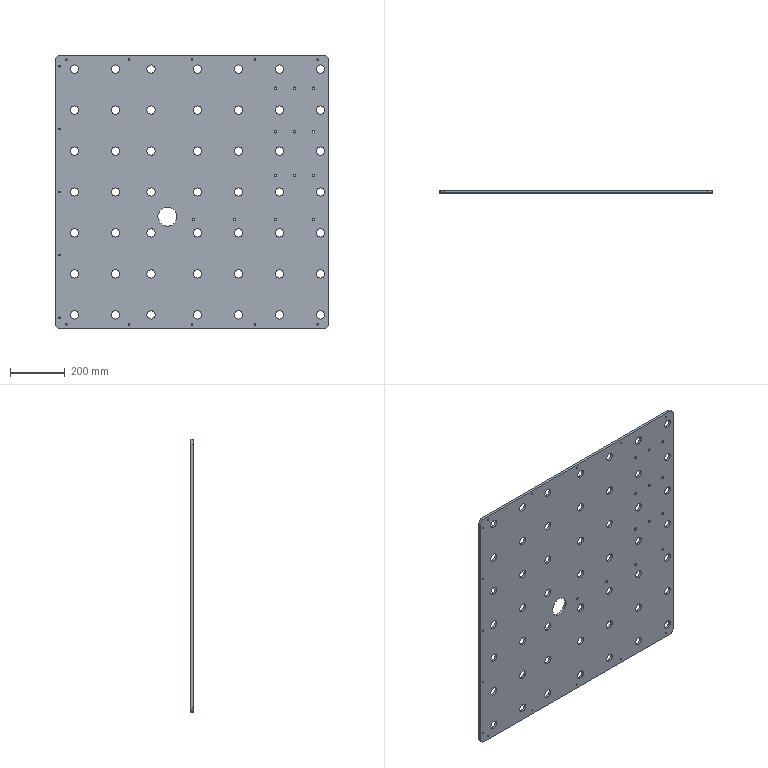Part | SolidWorks | 1 solid | 192 faces | box 1000 x 8 x 1000 mm | volume 7675541 mm3 | cylinder 160 | cone 26 | plane 6 | commonest cylinder face diameters 30 x98 5 x30 9 x26 40 x4 70 x2